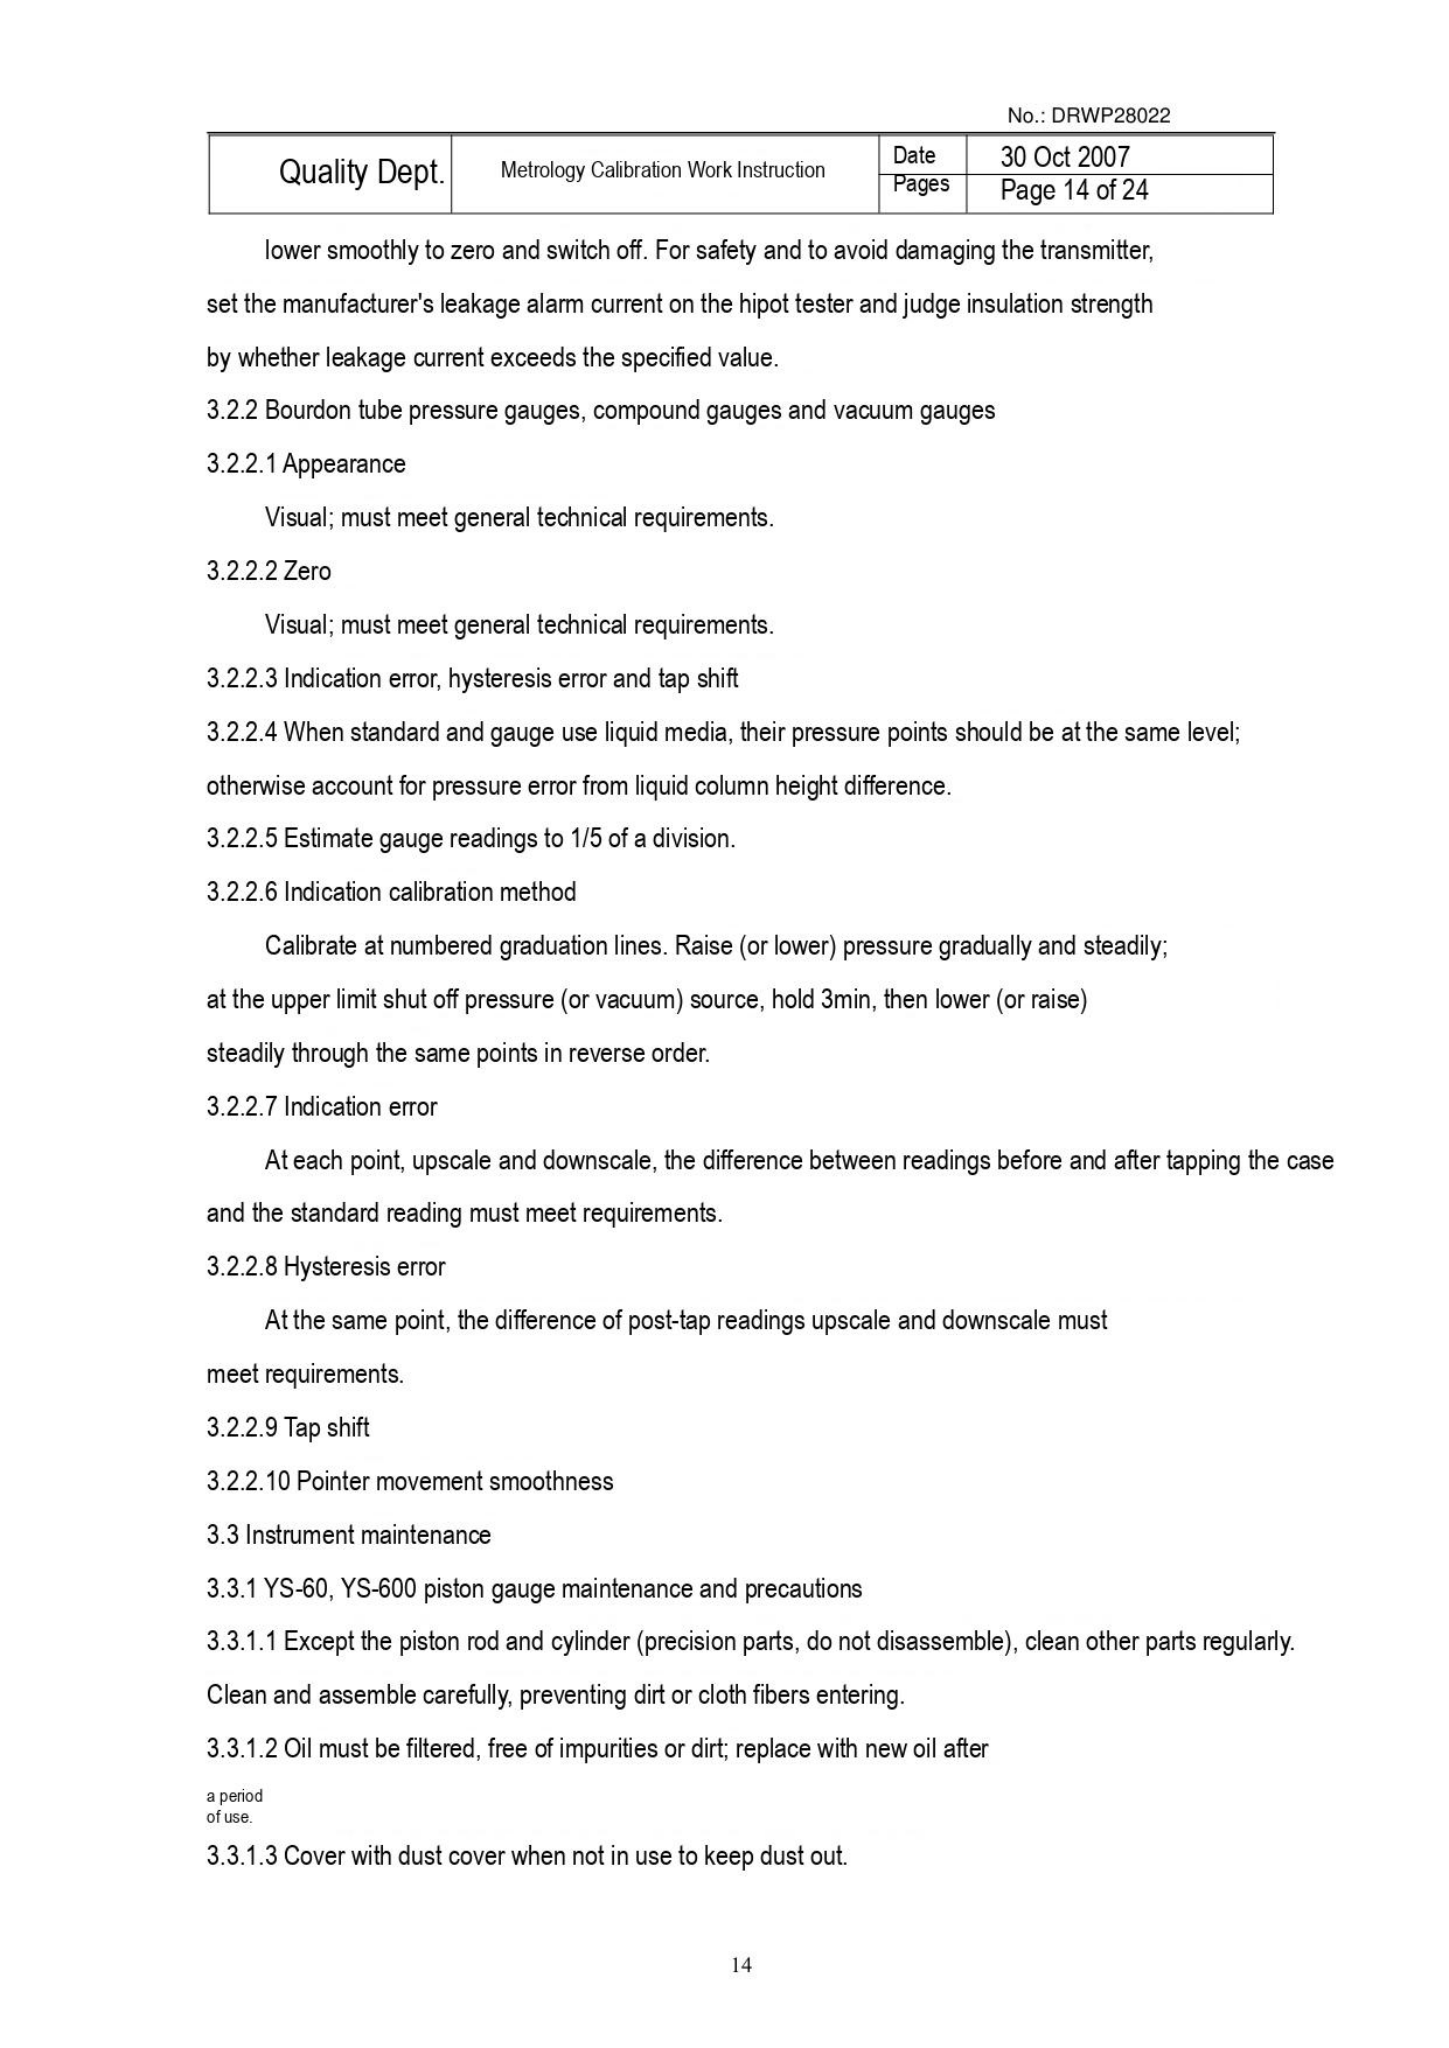No.: DRWP28022

| Quality Dept. | Metrology Calibration Work Instruction | Date | 30 Oct 2007 |
|---|---|---|---|
| | | Pages | Page 14 of 24 |

lower smoothly to zero and switch off. For safety and to avoid damaging the transmitter, set the manufacturer's leakage alarm current on the hipot tester and judge insulation strength by whether leakage current exceeds the specified value.

3.2.2 Bourdon tube pressure gauges, compound gauges and vacuum gauges

3.2.2.1 Appearance

Visual; must meet general technical requirements.

3.2.2.2 Zero

Visual; must meet general technical requirements.

3.2.2.3 Indication error, hysteresis error and tap shift

3.2.2.4 When standard and gauge use liquid media, their pressure points should be at the same level; otherwise account for pressure error from liquid column height difference.

3.2.2.5 Estimate gauge readings to 1/5 of a division.

3.2.2.6 Indication calibration method

Calibrate at numbered graduation lines. Raise (or lower) pressure gradually and steadily; at the upper limit shut off pressure (or vacuum) source, hold 3min, then lower (or raise) steadily through the same points in reverse order.

3.2.2.7 Indication error

At each point, upscale and downscale, the difference between readings before and after tapping the case and the standard reading must meet requirements.

3.2.2.8 Hysteresis error

At the same point, the difference of post-tap readings upscale and downscale must meet requirements.

3.2.2.9 Tap shift

3.2.2.10 Pointer movement smoothness

3.3 Instrument maintenance

3.3.1 YS-60, YS-600 piston gauge maintenance and precautions

3.3.1.1 Except the piston rod and cylinder (precision parts, do not disassemble), clean other parts regularly. Clean and assemble carefully, preventing dirt or cloth fibers entering.

3.3.1.2 Oil must be filtered, free of impurities or dirt; replace with new oil after a period of use.

3.3.1.3 Cover with dust cover when not in use to keep dust out.

14
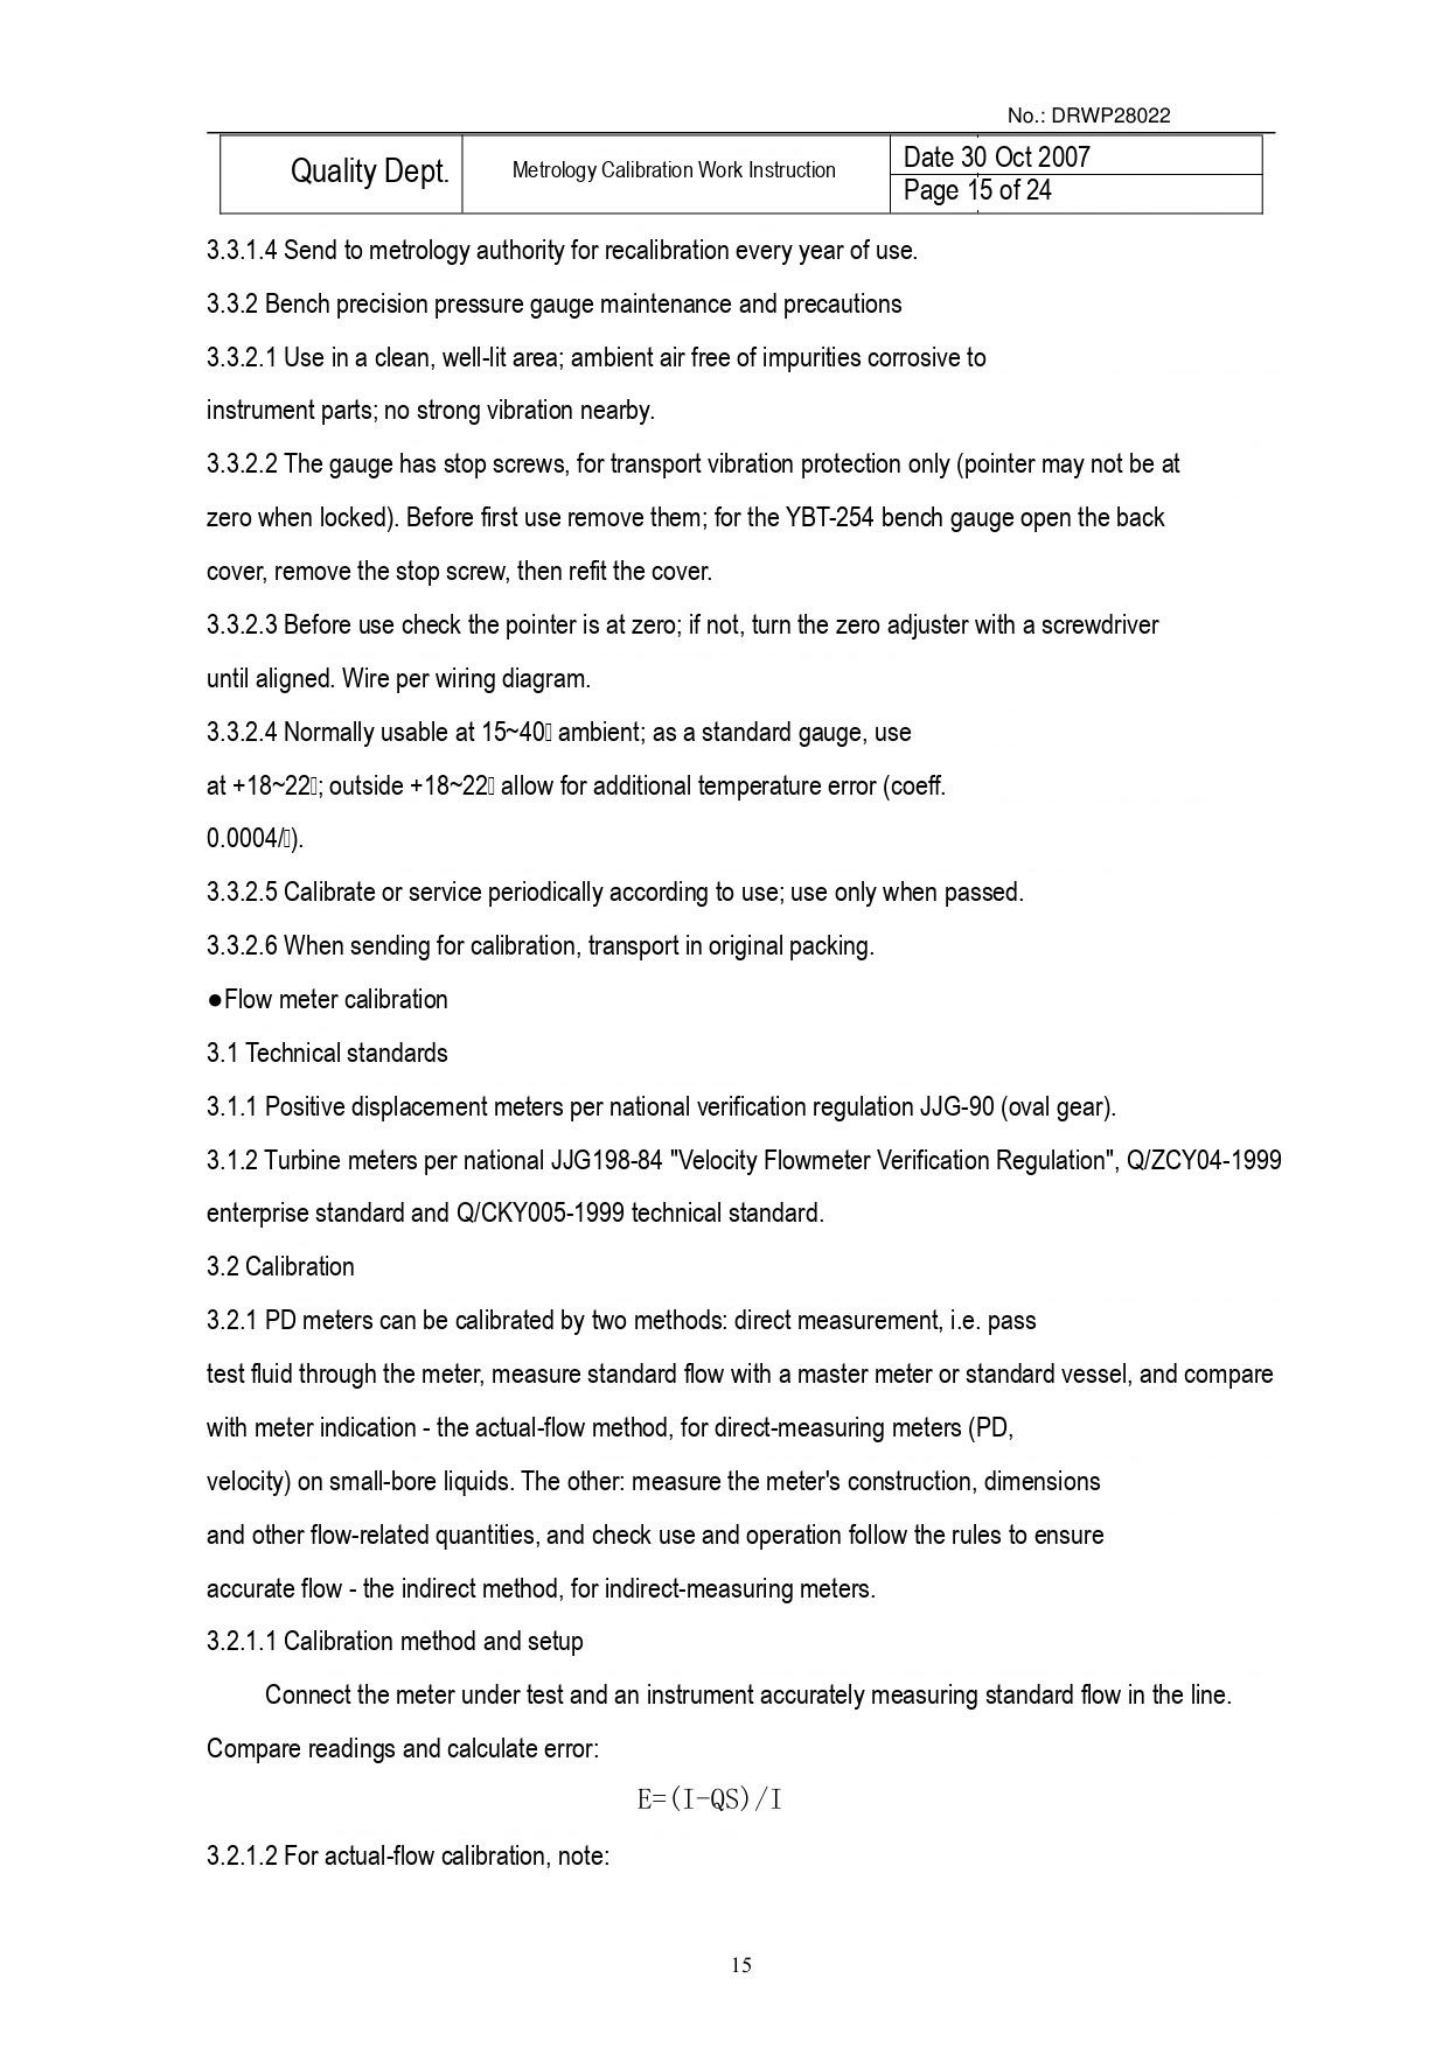No.: DRWP28022

| Quality Dept. | Metrology Calibration Work Instruction | Date 30 Oct 2007 |
|---|---|---|
| | | Page 15 of 24 |

3.3.1.4 Send to metrology authority for recalibration every year of use.

3.3.2 Bench precision pressure gauge maintenance and precautions

3.3.2.1 Use in a clean, well-lit area; ambient air free of impurities corrosive to instrument parts; no strong vibration nearby.

3.3.2.2 The gauge has stop screws, for transport vibration protection only (pointer may not be at zero when locked). Before first use remove them; for the YBT-254 bench gauge open the back cover, remove the stop screw, then refit the cover.

3.3.2.3 Before use check the pointer is at zero; if not, turn the zero adjuster with a screwdriver until aligned. Wire per wiring diagram.

3.3.2.4 Normally usable at 15~40 ambient; as a standard gauge, use at +18~22; outside +18~22 allow for additional temperature error (coeff. 0.0004/).

3.3.2.5 Calibrate or service periodically according to use; use only when passed.

3.3.2.6 When sending for calibration, transport in original packing.

●Flow meter calibration

3.1 Technical standards

3.1.1 Positive displacement meters per national verification regulation JJG-90 (oval gear).

3.1.2 Turbine meters per national JJG198-84 "Velocity Flowmeter Verification Regulation", Q/ZCY04-1999 enterprise standard and Q/CKY005-1999 technical standard.

3.2 Calibration

3.2.1 PD meters can be calibrated by two methods: direct measurement, i.e. pass test fluid through the meter, measure standard flow with a master meter or standard vessel, and compare with meter indication - the actual-flow method, for direct-measuring meters (PD, velocity) on small-bore liquids. The other: measure the meter's construction, dimensions and other flow-related quantities, and check use and operation follow the rules to ensure accurate flow - the indirect method, for indirect-measuring meters.

3.2.1.1 Calibration method and setup

Connect the meter under test and an instrument accurately measuring standard flow in the line. Compare readings and calculate error:

E=(I-QS)/I

3.2.1.2 For actual-flow calibration, note:

15
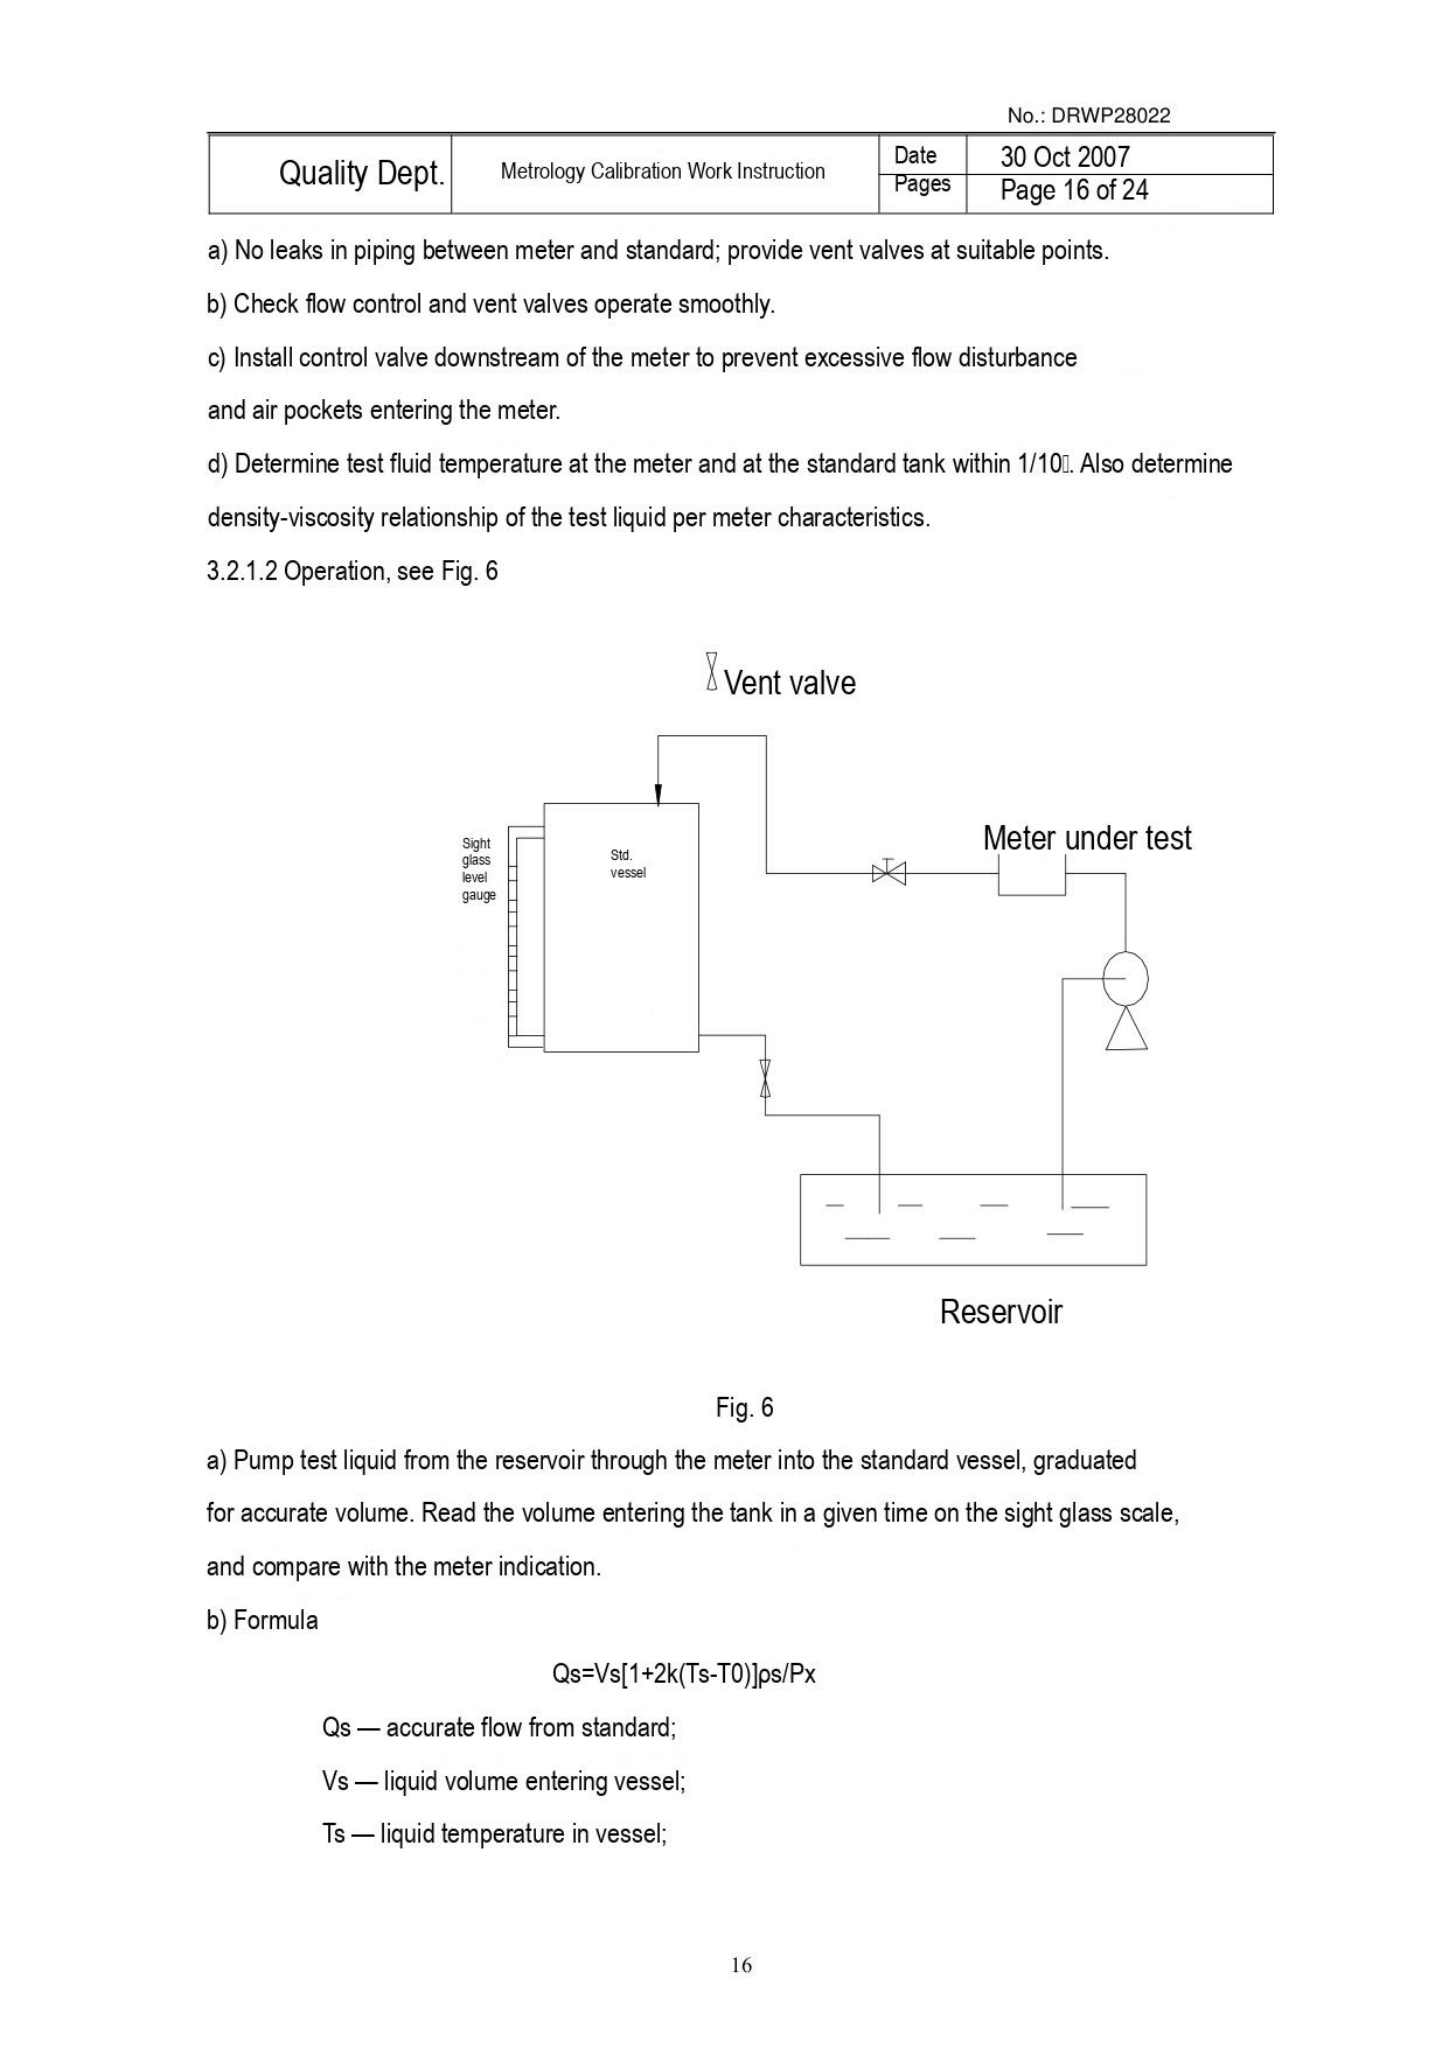No.: DRWP28022

| Quality Dept. | Metrology Calibration Work Instruction | Date | 30 Oct 2007 |
|---|---|---|---|
| | | Pages | Page 16 of 24 |

a) No leaks in piping between meter and standard; provide vent valves at suitable points.

b) Check flow control and vent valves operate smoothly.

c) Install control valve downstream of the meter to prevent excessive flow disturbance and air pockets entering the meter.

d) Determine test fluid temperature at the meter and at the standard tank within 1/10. Also determine density-viscosity relationship of the test liquid per meter characteristics.

3.2.1.2 Operation, see Fig. 6

Vent valve

Sight glass level gauge

Std. vessel

Meter under test

Reservoir

Fig. 6

a) Pump test liquid from the reservoir through the meter into the standard vessel, graduated for accurate volume. Read the volume entering the tank in a given time on the sight glass scale, and compare with the meter indication.

b) Formula

Qs=Vs[1+2k(Ts-T0)]ρs/Px

Qs — accurate flow from standard;

Vs — liquid volume entering vessel;

Ts — liquid temperature in vessel;

16
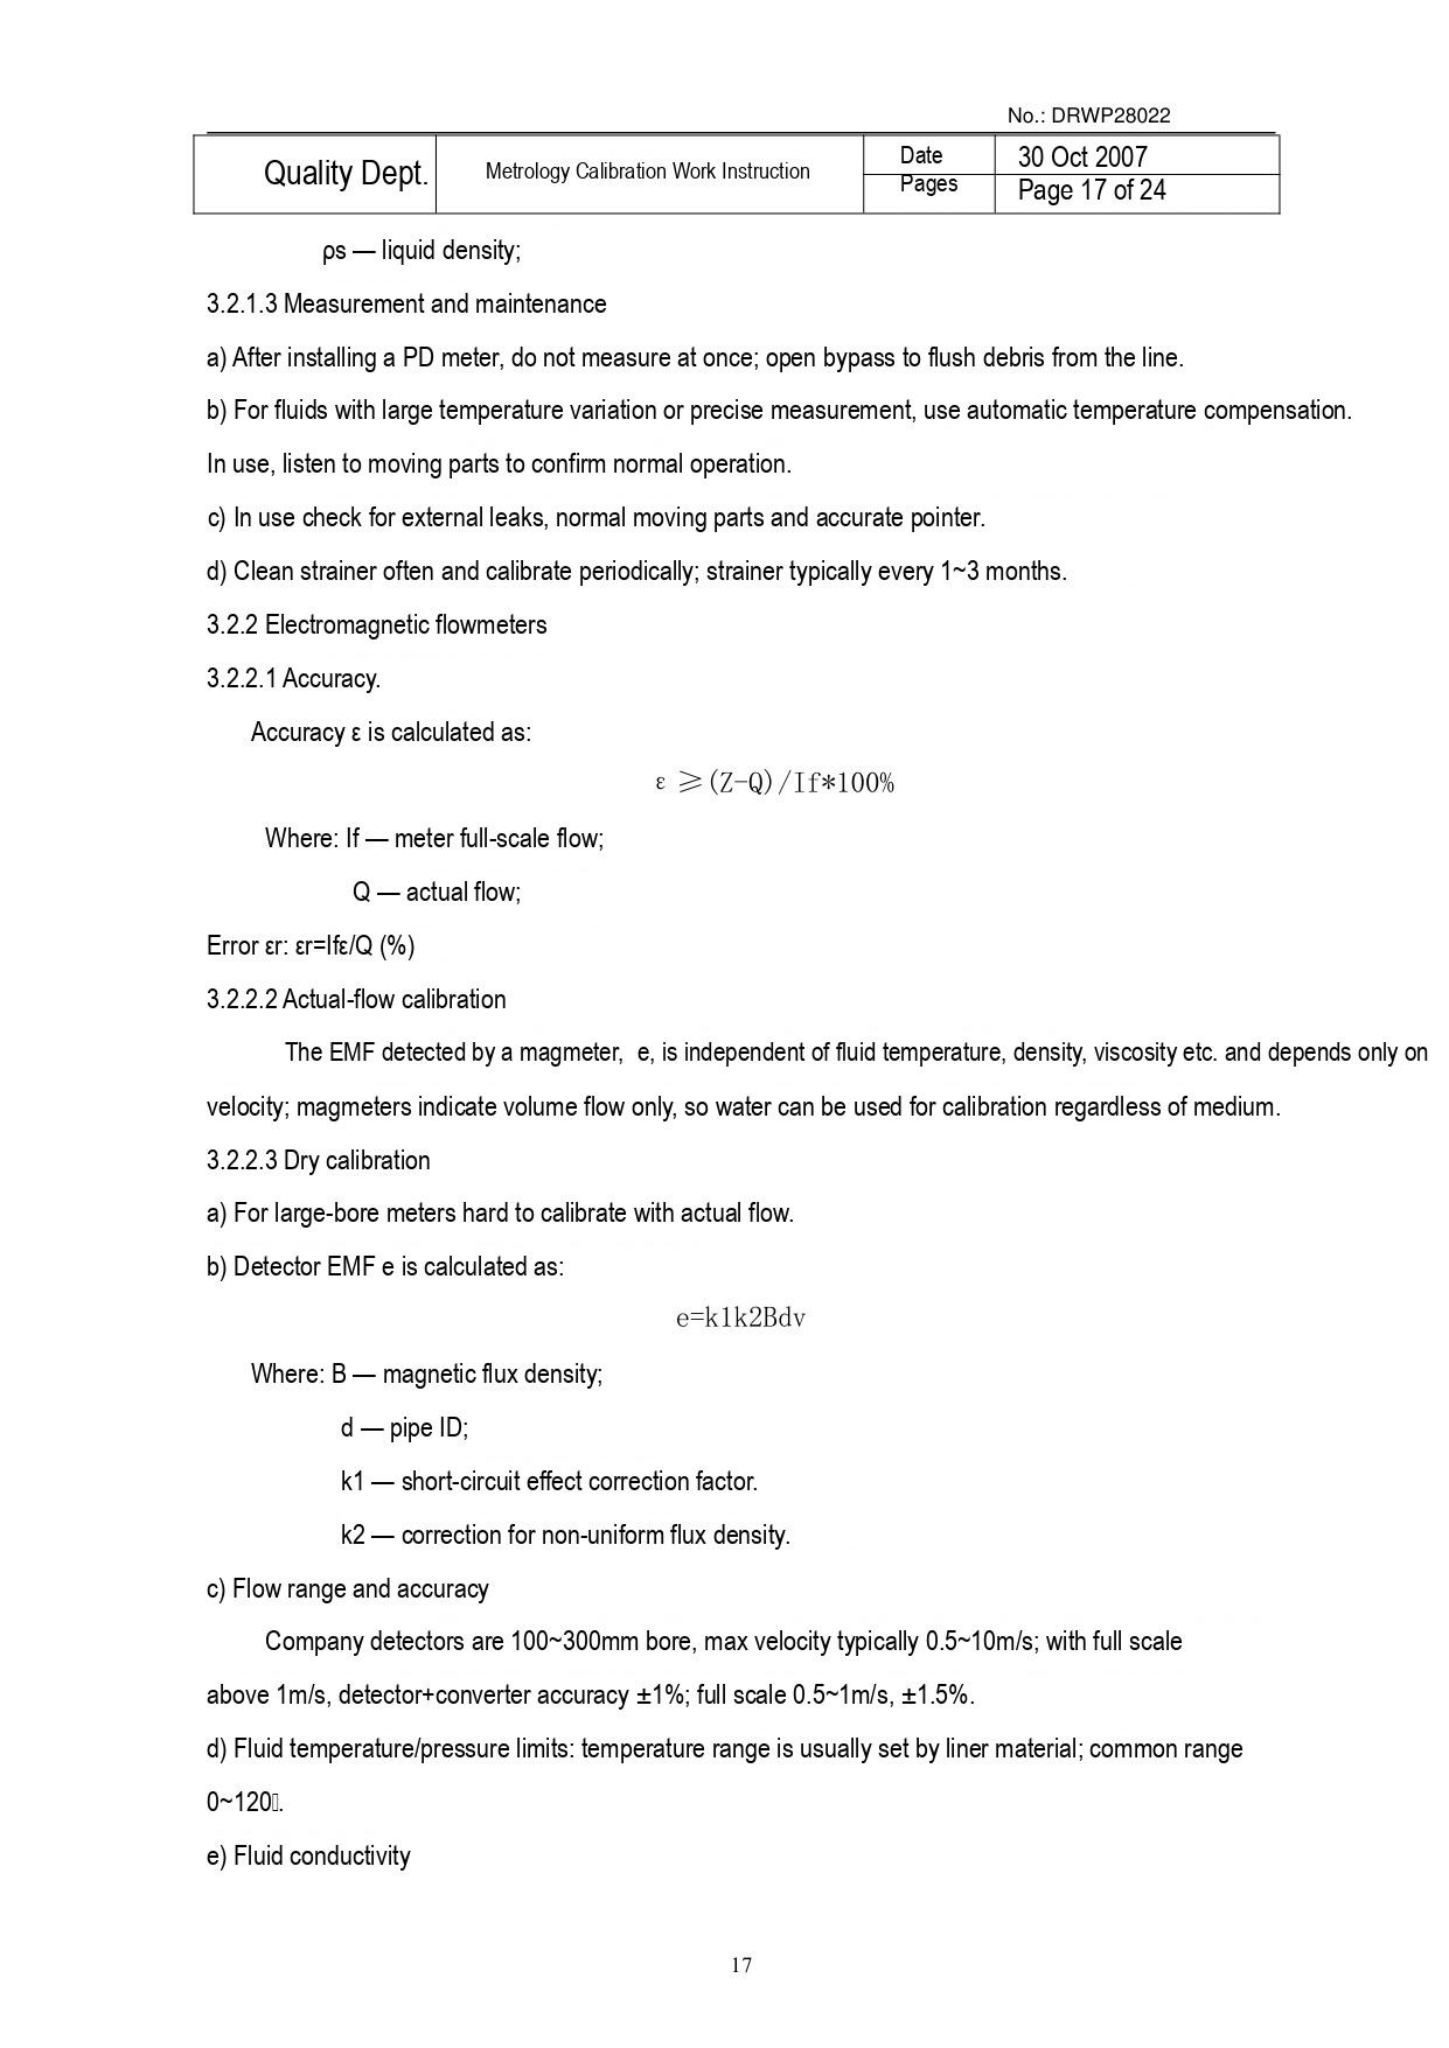No.: DRWP28022

| Quality Dept. | Metrology Calibration Work Instruction | Date | 30 Oct 2007 |
|---|---|---|---|
| | | Pages | Page 17 of 24 |

ρs — liquid density;

3.2.1.3 Measurement and maintenance

a) After installing a PD meter, do not measure at once; open bypass to flush debris from the line.

b) For fluids with large temperature variation or precise measurement, use automatic temperature compensation. In use, listen to moving parts to confirm normal operation.

c) In use check for external leaks, normal moving parts and accurate pointer.

d) Clean strainer often and calibrate periodically; strainer typically every 1~3 months.

3.2.2 Electromagnetic flowmeters

3.2.2.1 Accuracy.

Accuracy ε is calculated as:

ε ≥ (Z−Q) / If∗100%

Where: If — meter full-scale flow;

Q — actual flow;

Error εr: εr=Ifε/Q (%)

3.2.2.2 Actual-flow calibration

The EMF detected by a magmeter, e, is independent of fluid temperature, density, viscosity etc. and depends only on velocity; magmeters indicate volume flow only, so water can be used for calibration regardless of medium.

3.2.2.3 Dry calibration

a) For large-bore meters hard to calibrate with actual flow.

b) Detector EMF e is calculated as:

e=k1k2Bdv

Where: B — magnetic flux density;

d — pipe ID;

k1 — short-circuit effect correction factor.

k2 — correction for non-uniform flux density.

c) Flow range and accuracy

Company detectors are 100~300mm bore, max velocity typically 0.5~10m/s; with full scale above 1m/s, detector+converter accuracy ±1%; full scale 0.5~1m/s, ±1.5%.

d) Fluid temperature/pressure limits: temperature range is usually set by liner material; common range 0~120.

e) Fluid conductivity

17
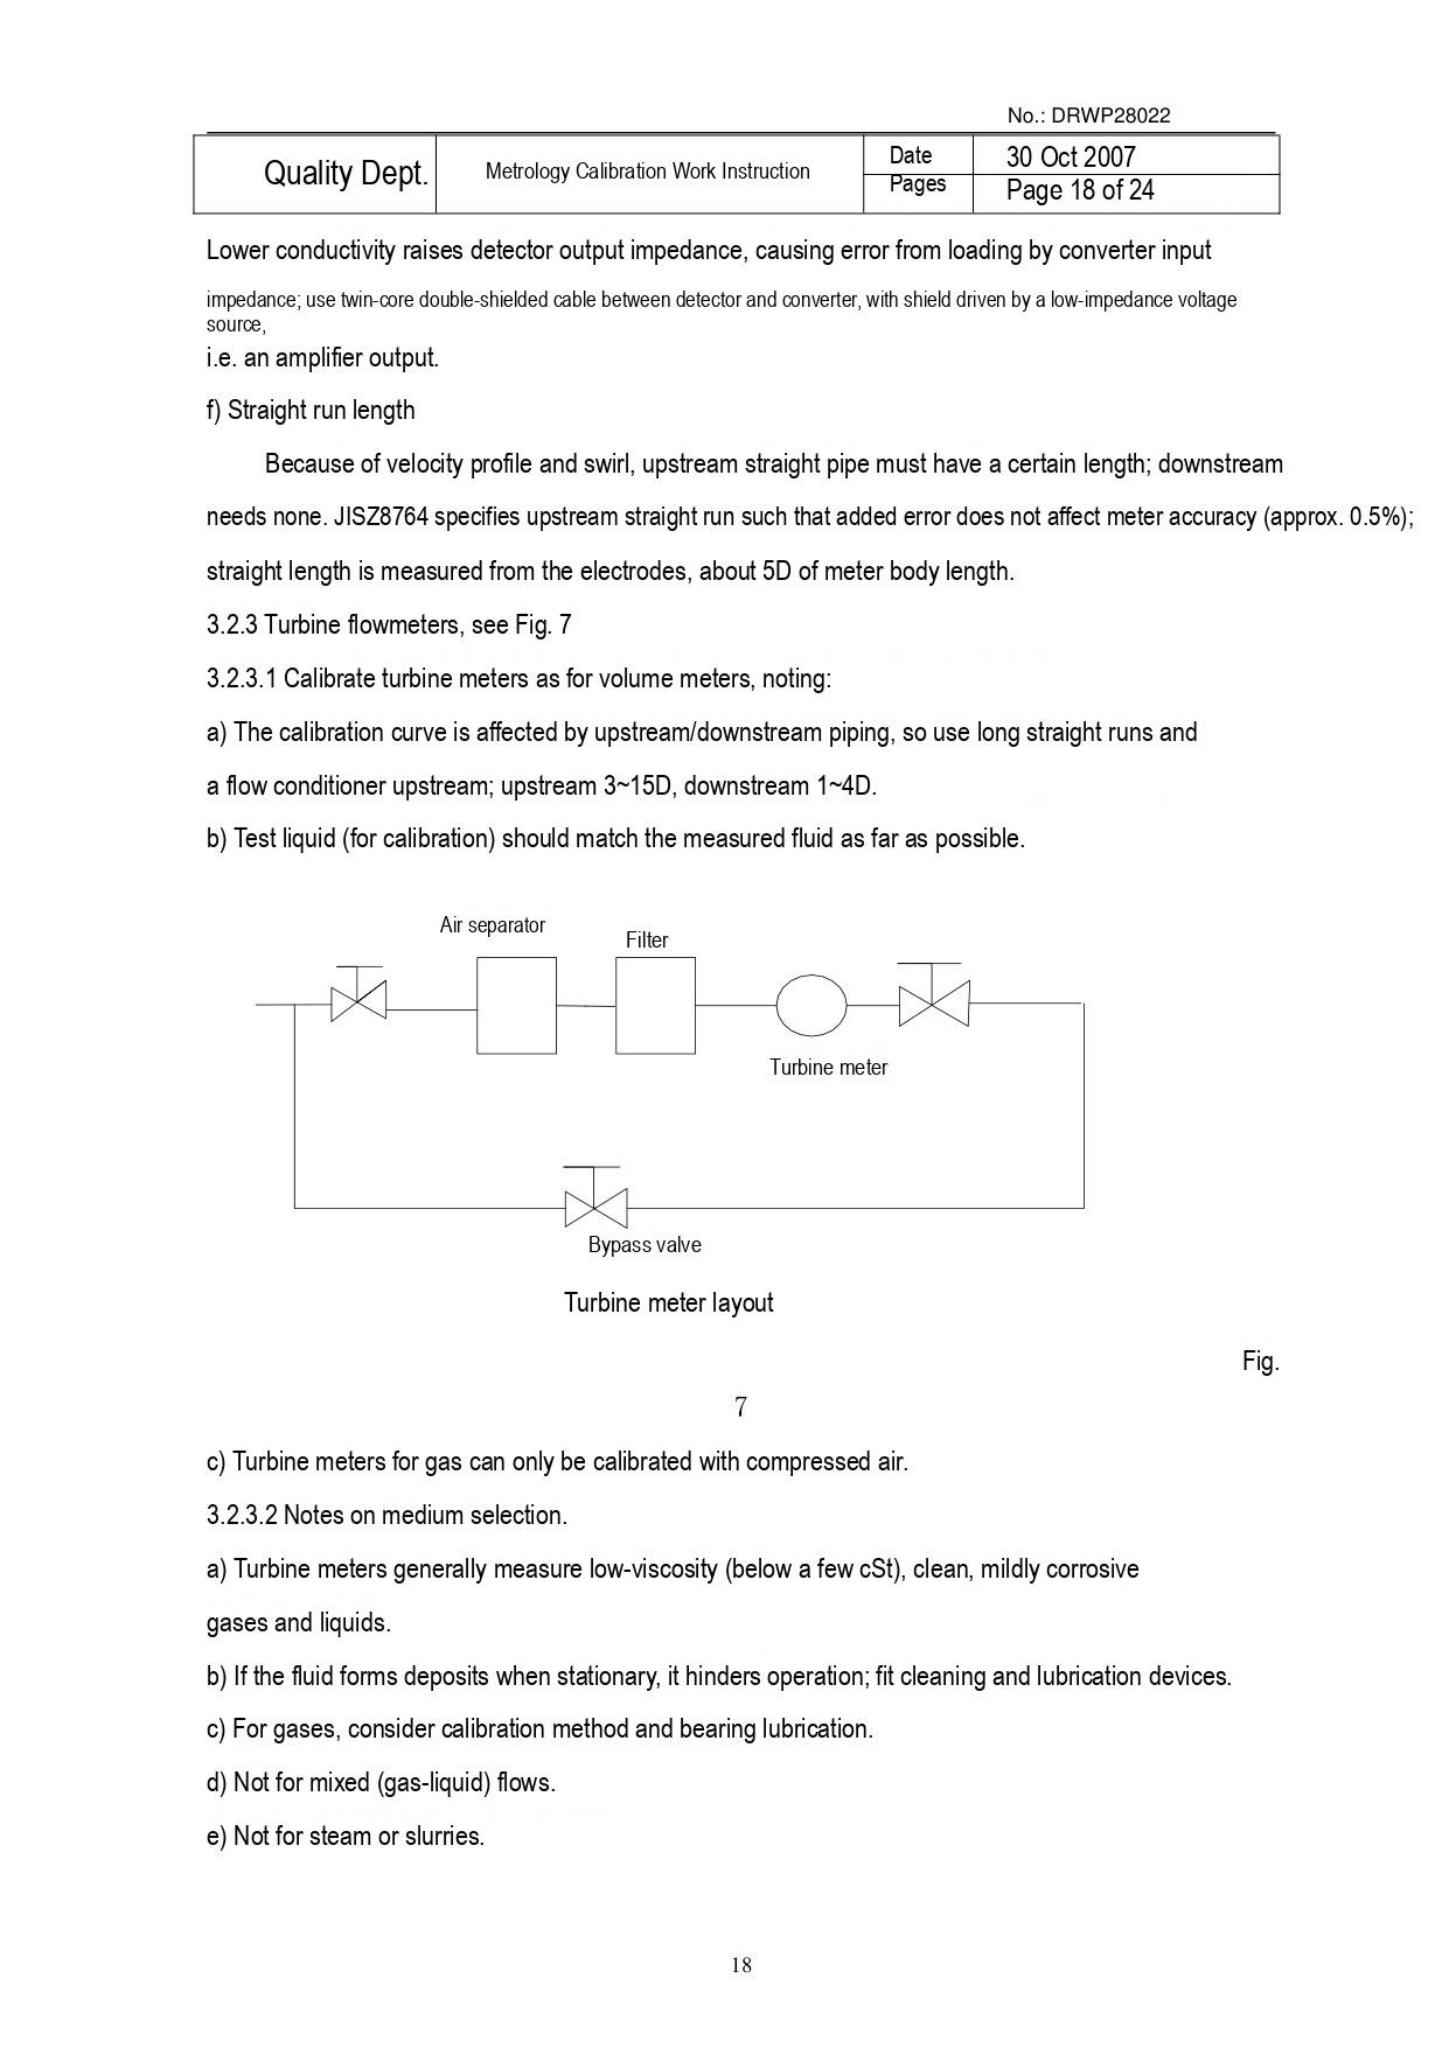No.: DRWP28022

| Quality Dept. | Metrology Calibration Work Instruction | Date | 30 Oct 2007 |
|---|---|---|---|
| | | Pages | Page 18 of 24 |

Lower conductivity raises detector output impedance, causing error from loading by converter input

impedance; use twin-core double-shielded cable between detector and converter, with shield driven by a low-impedance voltage source,

i.e. an amplifier output.

f) Straight run length

Because of velocity profile and swirl, upstream straight pipe must have a certain length; downstream needs none. JISZ8764 specifies upstream straight run such that added error does not affect meter accuracy (approx. 0.5%); straight length is measured from the electrodes, about 5D of meter body length.

3.2.3 Turbine flowmeters, see Fig. 7

3.2.3.1 Calibrate turbine meters as for volume meters, noting:

a) The calibration curve is affected by upstream/downstream piping, so use long straight runs and a flow conditioner upstream; upstream 3~15D, downstream 1~4D.

b) Test liquid (for calibration) should match the measured fluid as far as possible.

Air separator

Filter

Turbine meter

Bypass valve

Turbine meter layout

Fig.

7

c) Turbine meters for gas can only be calibrated with compressed air.

3.2.3.2 Notes on medium selection.

a) Turbine meters generally measure low-viscosity (below a few cSt), clean, mildly corrosive gases and liquids.

b) If the fluid forms deposits when stationary, it hinders operation; fit cleaning and lubrication devices.

c) For gases, consider calibration method and bearing lubrication.

d) Not for mixed (gas-liquid) flows.

e) Not for steam or slurries.

18
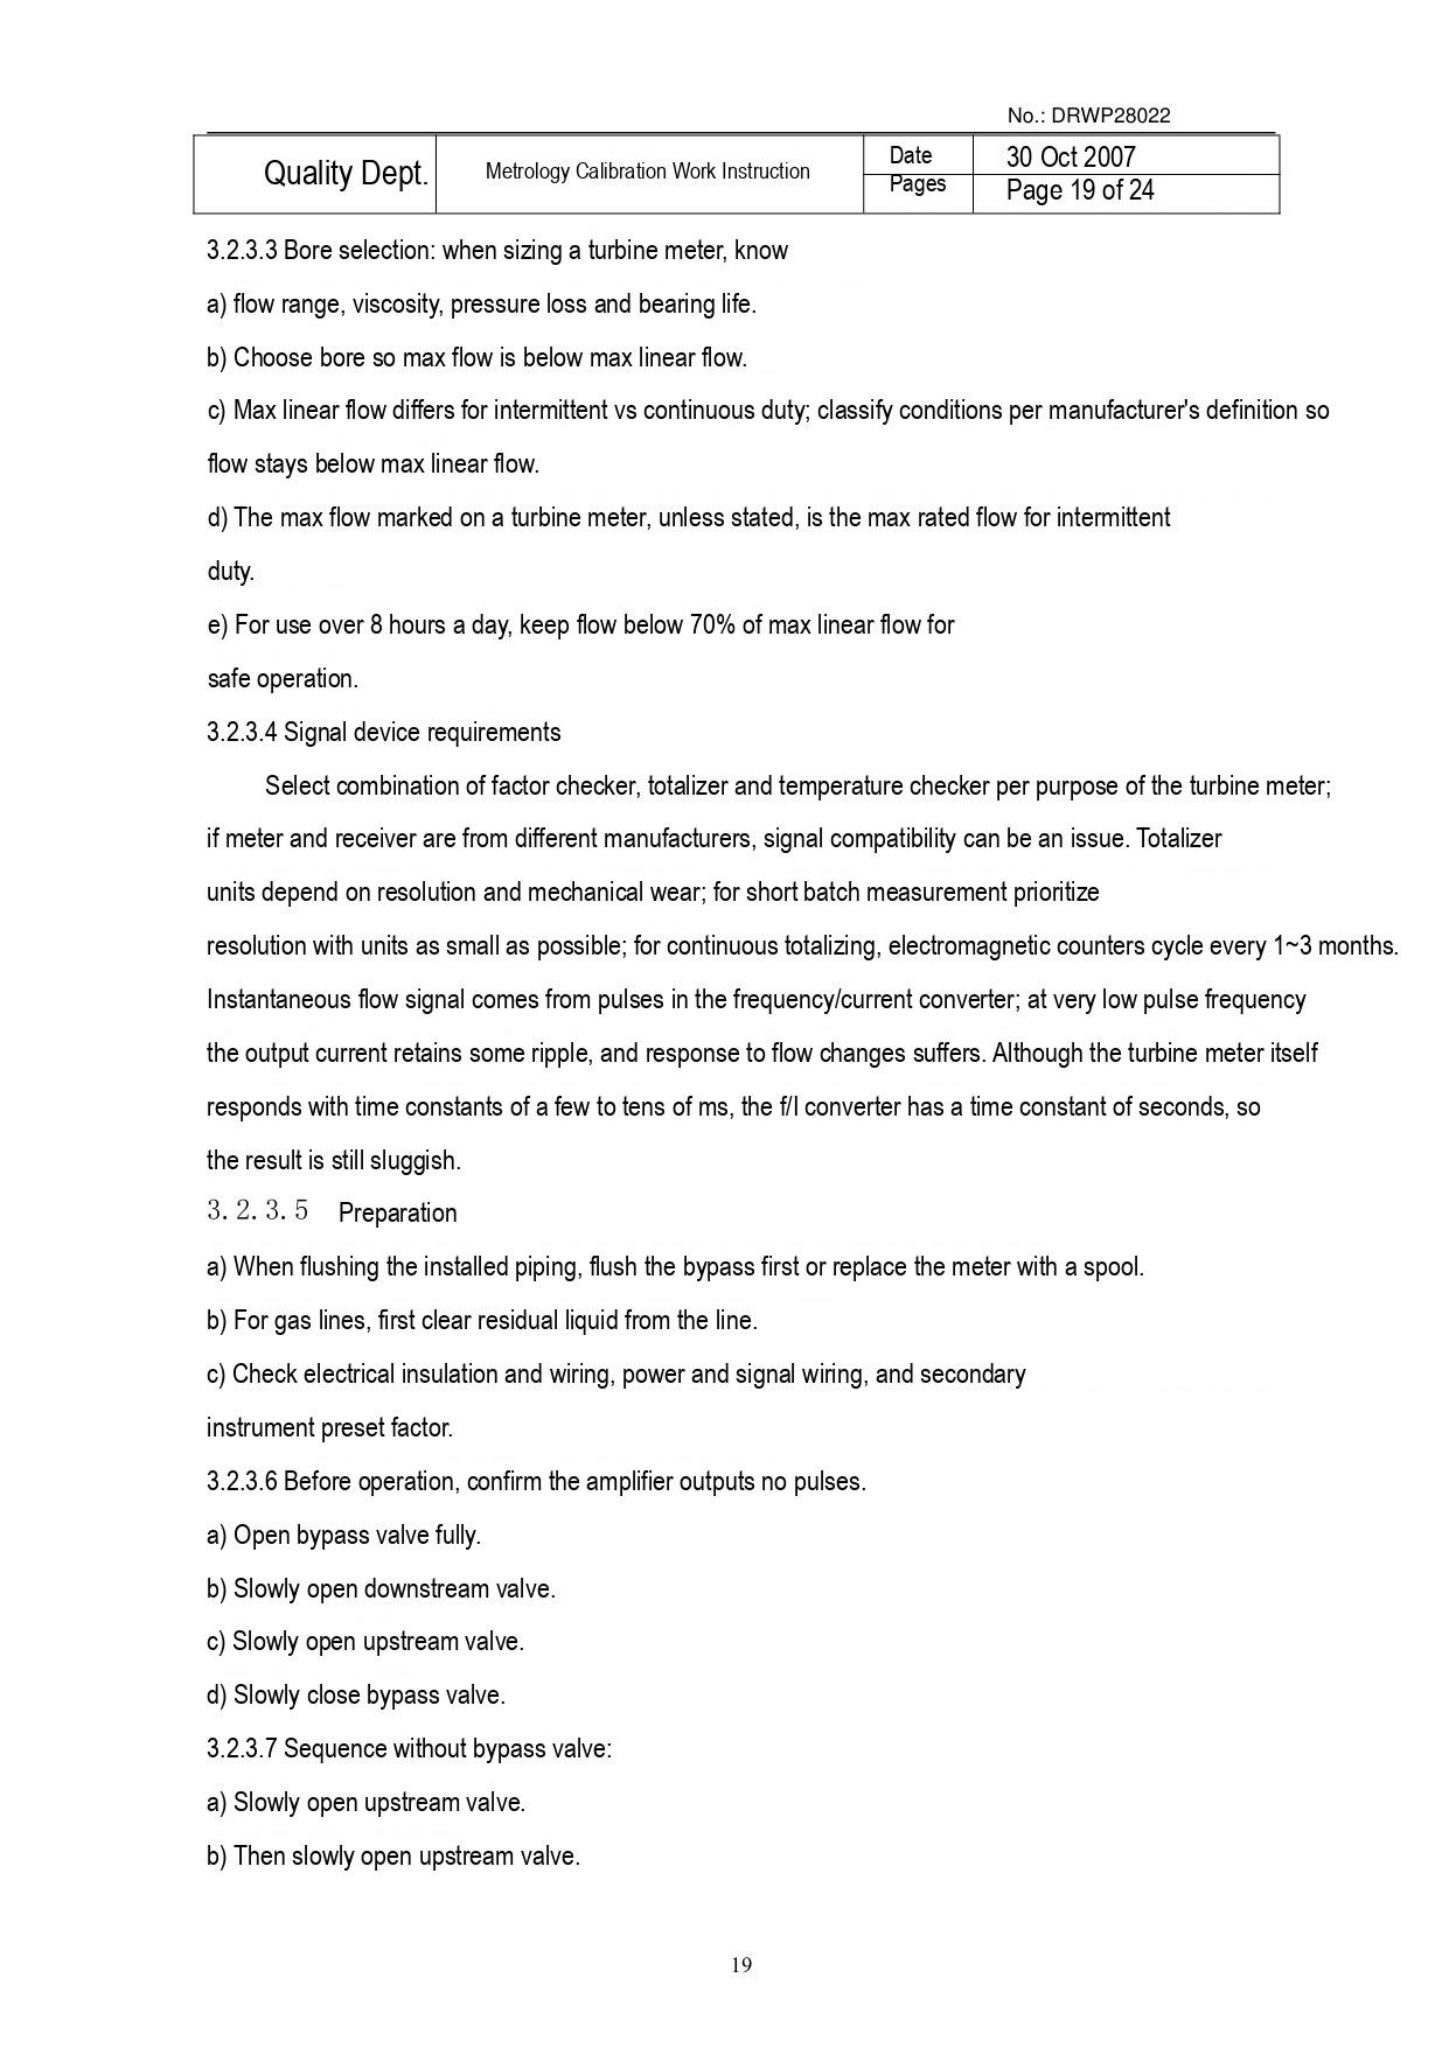No.: DRWP28022

| Quality Dept. | Metrology Calibration Work Instruction | Date | 30 Oct 2007 |
|---|---|---|---|
| | | Pages | Page 19 of 24 |

3.2.3.3 Bore selection: when sizing a turbine meter, know

a) flow range, viscosity, pressure loss and bearing life.

b) Choose bore so max flow is below max linear flow.

c) Max linear flow differs for intermittent vs continuous duty; classify conditions per manufacturer's definition so flow stays below max linear flow.

d) The max flow marked on a turbine meter, unless stated, is the max rated flow for intermittent duty.

e) For use over 8 hours a day, keep flow below 70% of max linear flow for safe operation.

3.2.3.4 Signal device requirements

Select combination of factor checker, totalizer and temperature checker per purpose of the turbine meter; if meter and receiver are from different manufacturers, signal compatibility can be an issue. Totalizer units depend on resolution and mechanical wear; for short batch measurement prioritize resolution with units as small as possible; for continuous totalizing, electromagnetic counters cycle every 1~3 months. Instantaneous flow signal comes from pulses in the frequency/current converter; at very low pulse frequency the output current retains some ripple, and response to flow changes suffers. Although the turbine meter itself responds with time constants of a few to tens of ms, the f/I converter has a time constant of seconds, so the result is still sluggish.

3.2.3.5 Preparation

a) When flushing the installed piping, flush the bypass first or replace the meter with a spool.

b) For gas lines, first clear residual liquid from the line.

c) Check electrical insulation and wiring, power and signal wiring, and secondary instrument preset factor.

3.2.3.6 Before operation, confirm the amplifier outputs no pulses.

a) Open bypass valve fully.

b) Slowly open downstream valve.

c) Slowly open upstream valve.

d) Slowly close bypass valve.

3.2.3.7 Sequence without bypass valve:

a) Slowly open upstream valve.

b) Then slowly open upstream valve.

19
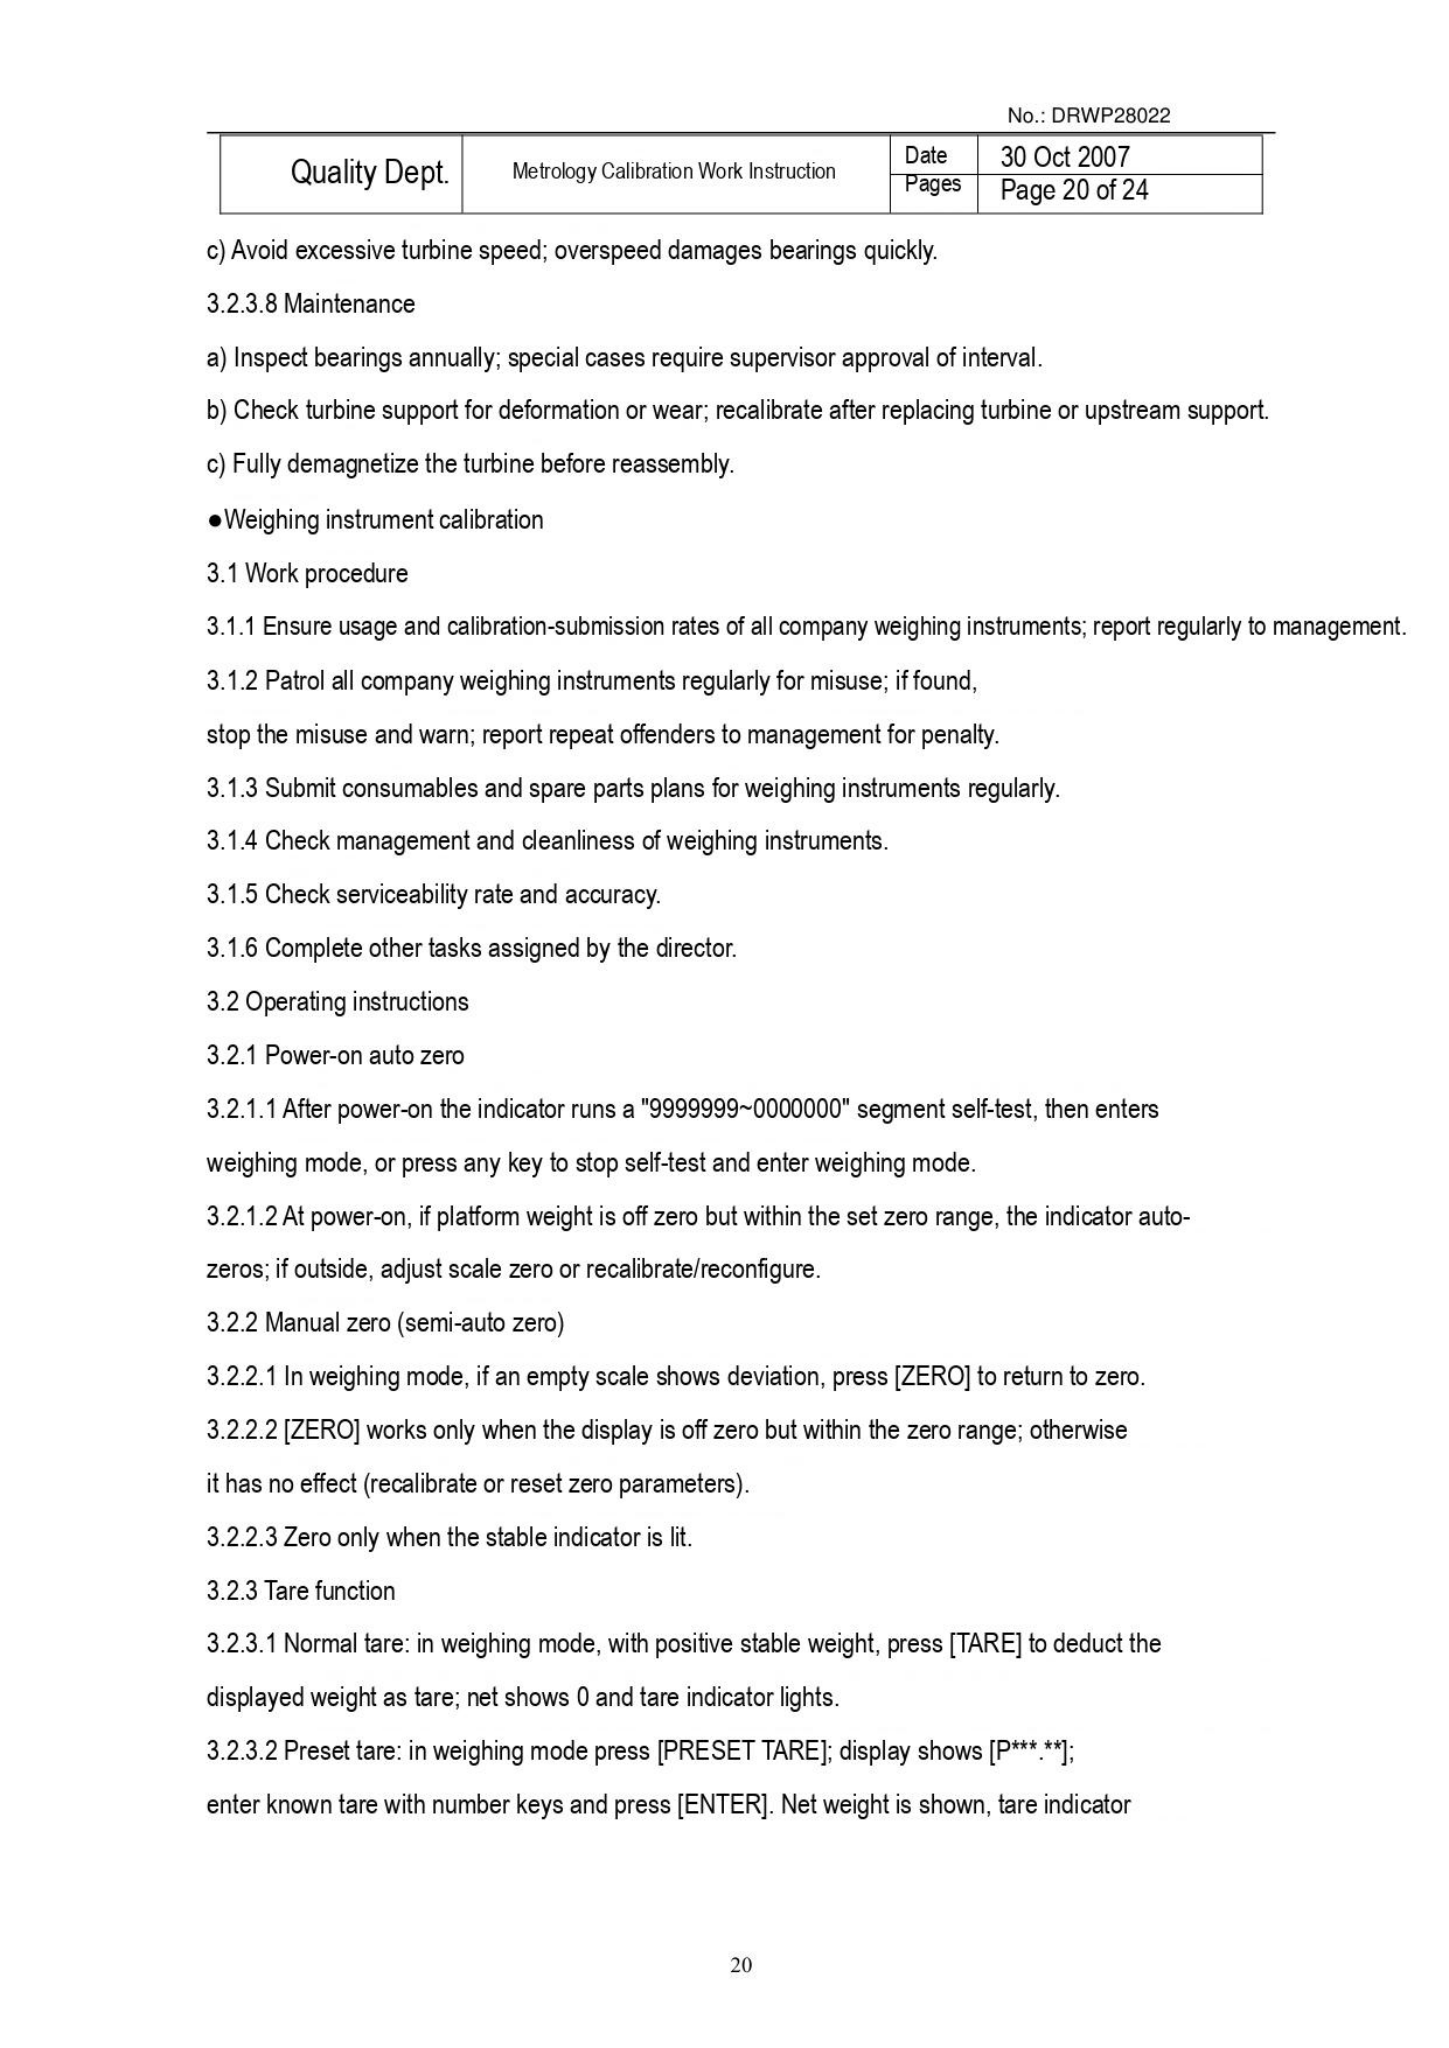No.: DRWP28022

| Quality Dept. | Metrology Calibration Work Instruction | Date | 30 Oct 2007 |
|---|---|---|---|
| | | Pages | Page 20 of 24 |

c) Avoid excessive turbine speed; overspeed damages bearings quickly.

3.2.3.8 Maintenance

a) Inspect bearings annually; special cases require supervisor approval of interval.

b) Check turbine support for deformation or wear; recalibrate after replacing turbine or upstream support.

c) Fully demagnetize the turbine before reassembly.

●Weighing instrument calibration

3.1 Work procedure

3.1.1 Ensure usage and calibration-submission rates of all company weighing instruments; report regularly to management.

3.1.2 Patrol all company weighing instruments regularly for misuse; if found,
stop the misuse and warn; report repeat offenders to management for penalty.

3.1.3 Submit consumables and spare parts plans for weighing instruments regularly.

3.1.4 Check management and cleanliness of weighing instruments.

3.1.5 Check serviceability rate and accuracy.

3.1.6 Complete other tasks assigned by the director.

3.2 Operating instructions

3.2.1 Power-on auto zero

3.2.1.1 After power-on the indicator runs a "9999999~0000000" segment self-test, then enters
weighing mode, or press any key to stop self-test and enter weighing mode.

3.2.1.2 At power-on, if platform weight is off zero but within the set zero range, the indicator auto-
zeros; if outside, adjust scale zero or recalibrate/reconfigure.

3.2.2 Manual zero (semi-auto zero)

3.2.2.1 In weighing mode, if an empty scale shows deviation, press [ZERO] to return to zero.

3.2.2.2 [ZERO] works only when the display is off zero but within the zero range; otherwise
it has no effect (recalibrate or reset zero parameters).

3.2.2.3 Zero only when the stable indicator is lit.

3.2.3 Tare function

3.2.3.1 Normal tare: in weighing mode, with positive stable weight, press [TARE] to deduct the
displayed weight as tare; net shows 0 and tare indicator lights.

3.2.3.2 Preset tare: in weighing mode press [PRESET TARE]; display shows [P***.**];
enter known tare with number keys and press [ENTER]. Net weight is shown, tare indicator

20